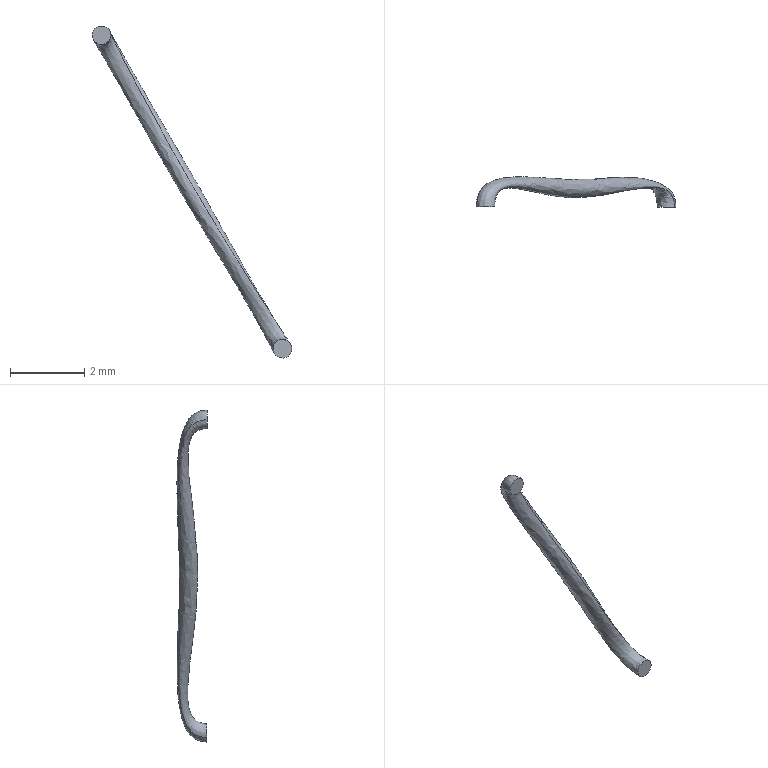Part | SolidWorks | features BaseBody 1 | 1 solid | 4 faces | box 5.38 x 0.8138 x 8.952 mm | volume 1.492 mm3 | plane 2 | spline 2
STEP:
#1=CARTESIAN_POINT('',(349.369,424.471,116.724));
#2=VERTEX_POINT('',#1);
#3=CARTESIAN_POINT('',(348.87,424.471,116.694));
#4=VERTEX_POINT('',#3);
#5=CARTESIAN_POINT('',(349.369,424.471,116.724));
#6=CARTESIAN_POINT('',(349.367,424.471,116.757));
#7=CARTESIAN_POINT('',(349.349,424.471,116.824));
#8=CARTESIAN_POINT('',(349.289,424.471,116.9));
#9=CARTESIAN_POINT('',(349.206,424.471,116.951));
#10=CARTESIAN_POINT('',(349.111,424.471,116.965));
#11=CARTESIAN_POINT('',(349.024,424.471,116.945));
#12=CARTESIAN_POINT('',(348.935,424.471,116.891));
#13=CARTESIAN_POINT('',(348.888,424.471,116.819));
#14=CARTESIAN_POINT('',(348.873,424.471,116.754));
#15=CARTESIAN_POINT('',(348.87,424.471,116.735));
#16=CARTESIAN_POINT('',(348.869,424.471,116.715));
#17=CARTESIAN_POINT('',(348.869,424.471,116.701));
#18=CARTESIAN_POINT('',(348.87,424.471,116.694));
#19=B_SPLINE_CURVE_WITH_KNOTS('',3,(#5,#6,#7,#8,#9,#10,#11,#12,#13,#14,#15,#16,#17,#18),.UNSPECIFIED.,.F.,.F.,(4,1,1,1,1,1,1,1,1,1,1,4),(0.,0.125,0.25,0.375,0.5,0.6,0.7,0.9,0.925,0.95,0.975,1.),.UNSPECIFIED.);
#20=EDGE_CURVE('',#2,#4,#19,.T.);
#21=ORIENTED_EDGE('',*,*,#20,.T.);
#22=CARTESIAN_POINT('',(348.87,424.471,116.694));
#23=CARTESIAN_POINT('',(348.87,424.471,116.687));
#24=CARTESIAN_POINT('',(348.872,424.471,116.674));
#25=CARTESIAN_POINT('',(348.875,424.471,116.654));
#26=CARTESIAN_POINT('',(348.88,424.471,116.634));
#27=CARTESIAN_POINT('',(348.903,424.471,116.572));
#28=CARTESIAN_POINT('',(348.958,424.471,116.506));
#29=CARTESIAN_POINT('',(349.053,424.471,116.464));
#30=CARTESIAN_POINT('',(349.142,424.471,116.454));
#31=CARTESIAN_POINT('',(349.234,424.471,116.479));
#32=CARTESIAN_POINT('',(349.311,424.471,116.539));
#33=CARTESIAN_POINT('',(349.361,424.471,116.623));
#34=CARTESIAN_POINT('',(349.371,424.471,116.69));
#35=CARTESIAN_POINT('',(349.369,424.471,116.724));
#36=B_SPLINE_CURVE_WITH_KNOTS('',3,(#22,#23,#24,#25,#26,#27,#28,#29,#30,#31,#32,#33,#34,#35),.UNSPECIFIED.,.F.,.F.,(4,1,1,1,1,1,1,1,1,1,1,4),(0.,0.025,0.05,0.075,0.1,0.3,0.4,0.5,0.625,0.75,0.875,1.),.UNSPECIFIED.);
#37=EDGE_CURVE('',#4,#2,#36,.T.);
#38=ORIENTED_EDGE('',*,*,#37,.T.);
#39=EDGE_LOOP('',(#21,#38));
#40=FACE_OUTER_BOUND('',#39,.T.);
#41=CARTESIAN_POINT('',(349.119,424.471,116.709));
#42=DIRECTION('',(-0.0009599,1.,0.));
#43=DIRECTION('',(0.,0.,1.));
#44=AXIS2_PLACEMENT_3D('',#41,#42,#43);
#45=PLANE('',#44);
#46=ADVANCED_FACE('',(#40),#45,.F.);
#47=CARTESIAN_POINT('',(354.216,424.476,108.382));
#48=VERTEX_POINT('',#47);
#49=CARTESIAN_POINT('',(353.783,424.475,108.132));
#50=VERTEX_POINT('',#49);
#51=CARTESIAN_POINT('',(354.216,424.476,108.382));
#52=CARTESIAN_POINT('',(354.199,424.476,108.411));
#53=CARTESIAN_POINT('',(354.153,424.476,108.462));
#54=CARTESIAN_POINT('',(354.065,424.476,108.504));
#55=CARTESIAN_POINT('',(353.968,424.476,108.512));
#56=CARTESIAN_POINT('',(353.877,424.476,108.482));
#57=CARTESIAN_POINT('',(353.809,424.475,108.425));
#58=CARTESIAN_POINT('',(353.753,424.475,108.337));
#59=CARTESIAN_POINT('',(353.743,424.475,108.251));
#60=CARTESIAN_POINT('',(353.759,424.475,108.188));
#61=CARTESIAN_POINT('',(353.765,424.475,108.169));
#62=CARTESIAN_POINT('',(353.773,424.475,108.15));
#63=CARTESIAN_POINT('',(353.779,424.475,108.138));
#64=CARTESIAN_POINT('',(353.783,424.475,108.132));
#65=B_SPLINE_CURVE_WITH_KNOTS('',3,(#51,#52,#53,#54,#55,#56,#57,#58,#59,#60,#61,#62,#63,#64),.UNSPECIFIED.,.F.,.F.,(4,1,1,1,1,1,1,1,1,1,1,4),(0.,0.125,0.25,0.375,0.5,0.6,0.7,0.9,0.925,0.95,0.975,1.),.UNSPECIFIED.);
#66=EDGE_CURVE('',#48,#50,#65,.T.);
#67=ORIENTED_EDGE('',*,*,#66,.T.);
#68=CARTESIAN_POINT('',(353.783,424.475,108.132));
#69=CARTESIAN_POINT('',(353.786,424.475,108.126));
#70=CARTESIAN_POINT('',(353.794,424.475,108.114));
#71=CARTESIAN_POINT('',(353.806,424.475,108.098));
#72=CARTESIAN_POINT('',(353.819,424.475,108.083));
#73=CARTESIAN_POINT('',(353.866,424.476,108.038));
#74=CARTESIAN_POINT('',(353.946,424.476,108.003));
#75=CARTESIAN_POINT('',(354.05,424.476,108.008));
#76=CARTESIAN_POINT('',(354.133,424.476,108.039));
#77=CARTESIAN_POINT('',(354.204,424.476,108.103));
#78=CARTESIAN_POINT('',(354.246,424.476,108.191));
#79=CARTESIAN_POINT('',(354.254,424.476,108.288));
#80=CARTESIAN_POINT('',(354.233,424.476,108.353));
#81=CARTESIAN_POINT('',(354.216,424.476,108.382));
#82=B_SPLINE_CURVE_WITH_KNOTS('',3,(#68,#69,#70,#71,#72,#73,#74,#75,#76,#77,#78,#79,#80,#81),.UNSPECIFIED.,.F.,.F.,(4,1,1,1,1,1,1,1,1,1,1,4),(0.,0.025,0.05,0.075,0.1,0.3,0.4,0.5,0.625,0.75,0.875,1.),.UNSPECIFIED.);
#83=EDGE_CURVE('',#50,#48,#82,.T.);
#84=ORIENTED_EDGE('',*,*,#83,.T.);
#85=EDGE_LOOP('',(#67,#84));
#86=FACE_OUTER_BOUND('',#85,.T.);
#87=CARTESIAN_POINT('',(353.999,424.476,108.257));
#88=DIRECTION('',(-0.0009599,1.,0.));
#89=DIRECTION('',(0.,0.,1.));
#90=AXIS2_PLACEMENT_3D('',#87,#88,#89);
#91=PLANE('',#90);
#92=ADVANCED_FACE('',(#86),#91,.F.);
#93=CARTESIAN_POINT('',(354.216,424.476,108.382));
#94=CARTESIAN_POINT('',(354.215,425.491,108.382));
#95=CARTESIAN_POINT('',(351.494,424.025,112.508));
#96=CARTESIAN_POINT('',(349.368,425.464,116.724));
#97=CARTESIAN_POINT('',(349.369,424.471,116.724));
#98=B_SPLINE_CURVE_WITH_KNOTS('',3,(#93,#94,#95,#96,#97),.UNSPECIFIED.,.F.,.F.,(4,1,4),(0.,0.5001,1.),.UNSPECIFIED.);
#99=EDGE_CURVE('',#48,#2,#98,.T.);
#100=ORIENTED_EDGE('',*,*,#99,.T.);
#101=ORIENTED_EDGE('',*,*,#37,.F.);
#102=CARTESIAN_POINT('',(348.87,424.471,116.694));
#103=CARTESIAN_POINT('',(348.869,425.576,116.694));
#104=CARTESIAN_POINT('',(351.562,424.823,112.419));
#105=CARTESIAN_POINT('',(353.782,425.559,108.132));
#106=CARTESIAN_POINT('',(353.783,424.475,108.132));
#107=B_SPLINE_CURVE_WITH_KNOTS('',3,(#102,#103,#104,#105,#106),.UNSPECIFIED.,.F.,.F.,(4,1,4),(0.,0.4999,1.),.UNSPECIFIED.);
#108=EDGE_CURVE('',#4,#50,#107,.T.);
#109=ORIENTED_EDGE('',*,*,#108,.T.);
#110=ORIENTED_EDGE('',*,*,#66,.F.);
#111=EDGE_LOOP('',(#100,#101,#109,#110));
#112=FACE_OUTER_BOUND('',#111,.T.);
#113=CARTESIAN_POINT('',(354.219,424.375,108.374));
#114=CARTESIAN_POINT('',(354.307,425.541,108.239));
#115=CARTESIAN_POINT('',(351.502,423.989,112.524));
#116=CARTESIAN_POINT('',(349.295,425.516,116.88));
#117=CARTESIAN_POINT('',(349.371,424.365,116.732));
#118=CARTESIAN_POINT('',(354.217,424.375,108.379));
#119=CARTESIAN_POINT('',(354.304,425.54,108.244));
#120=CARTESIAN_POINT('',(351.495,423.985,112.52));
#121=CARTESIAN_POINT('',(349.296,425.515,116.875));
#122=CARTESIAN_POINT('',(349.372,424.366,116.727));
#123=CARTESIAN_POINT('',(354.198,424.376,108.413));
#124=CARTESIAN_POINT('',(354.287,425.531,108.28));
#125=CARTESIAN_POINT('',(351.443,423.956,112.488));
#126=CARTESIAN_POINT('',(349.301,425.506,116.836));
#127=CARTESIAN_POINT('',(349.375,424.366,116.689));
#128=CARTESIAN_POINT('',(354.149,424.378,108.468));
#129=CARTESIAN_POINT('',(354.24,425.515,108.339));
#130=CARTESIAN_POINT('',(351.348,423.93,112.424));
#131=CARTESIAN_POINT('',(349.293,425.494,116.763));
#132=CARTESIAN_POINT('',(349.365,424.368,116.616));
#133=CARTESIAN_POINT('',(354.061,424.379,108.51));
#134=CARTESIAN_POINT('',(354.152,425.5,108.384));
#135=CARTESIAN_POINT('',(351.248,423.966,112.346));
#136=CARTESIAN_POINT('',(349.245,425.485,116.679));
#137=CARTESIAN_POINT('',(349.314,424.369,116.532));
#138=CARTESIAN_POINT('',(353.964,424.38,108.517));
#139=CARTESIAN_POINT('',(354.054,425.492,108.394));
#140=CARTESIAN_POINT('',(351.187,424.062,112.285));
#141=CARTESIAN_POINT('',(349.167,425.486,116.62));
#142=CARTESIAN_POINT('',(349.237,424.368,116.472));
#143=CARTESIAN_POINT('',(353.874,424.379,108.487));
#144=CARTESIAN_POINT('',(353.96,425.493,108.364));
#145=CARTESIAN_POINT('',(351.177,424.205,112.252));
#146=CARTESIAN_POINT('',(349.072,425.495,116.595));
#147=CARTESIAN_POINT('',(349.145,424.367,116.447));
#148=CARTESIAN_POINT('',(353.805,424.378,108.431));
#149=CARTESIAN_POINT('',(353.888,425.503,108.306));
#150=CARTESIAN_POINT('',(351.211,424.361,112.249));
#151=CARTESIAN_POINT('',(348.98,425.513,116.605));
#152=CARTESIAN_POINT('',(349.057,424.365,116.456));
#153=CARTESIAN_POINT('',(353.75,424.376,108.343));
#154=CARTESIAN_POINT('',(353.829,425.524,108.215));
#155=CARTESIAN_POINT('',(351.293,424.544,112.274));
#156=CARTESIAN_POINT('',(348.879,425.541,116.648));
#157=CARTESIAN_POINT('',(348.962,424.362,116.499));
#158=CARTESIAN_POINT('',(353.74,424.373,108.257));
#159=CARTESIAN_POINT('',(353.815,425.547,108.124));
#160=CARTESIAN_POINT('',(351.395,424.675,112.324));
#161=CARTESIAN_POINT('',(348.818,425.567,116.715));
#162=CARTESIAN_POINT('',(348.907,424.359,116.565));
#163=CARTESIAN_POINT('',(353.755,424.371,108.194));
#164=CARTESIAN_POINT('',(353.829,425.565,108.057));
#165=CARTESIAN_POINT('',(351.484,424.747,112.374));
#166=CARTESIAN_POINT('',(348.792,425.586,116.777));
#167=CARTESIAN_POINT('',(348.885,424.356,116.627));
#168=CARTESIAN_POINT('',(353.762,424.371,108.175));
#169=CARTESIAN_POINT('',(353.834,425.571,108.037));
#170=CARTESIAN_POINT('',(351.511,424.767,112.39));
#171=CARTESIAN_POINT('',(348.786,425.591,116.796));
#172=CARTESIAN_POINT('',(348.88,424.356,116.646));
#173=CARTESIAN_POINT('',(353.77,424.37,108.156));
#174=CARTESIAN_POINT('',(353.842,425.576,108.017));
#175=CARTESIAN_POINT('',(351.539,424.784,112.406));
#176=CARTESIAN_POINT('',(348.781,425.596,116.816));
#177=CARTESIAN_POINT('',(348.876,424.355,116.666));
#178=CARTESIAN_POINT('',(353.779,424.37,108.14));
#179=CARTESIAN_POINT('',(353.85,425.581,108.));
#180=CARTESIAN_POINT('',(351.564,424.798,112.422));
#181=CARTESIAN_POINT('',(348.779,425.601,116.835));
#182=CARTESIAN_POINT('',(348.874,424.355,116.685));
#183=CARTESIAN_POINT('',(353.785,424.37,108.129));
#184=CARTESIAN_POINT('',(353.856,425.585,107.989));
#185=CARTESIAN_POINT('',(351.581,424.806,112.433));
#186=CARTESIAN_POINT('',(348.778,425.604,116.847));
#187=CARTESIAN_POINT('',(348.874,424.355,116.697));
#188=CARTESIAN_POINT('',(353.788,424.369,108.125));
#189=CARTESIAN_POINT('',(353.859,425.586,107.984));
#190=CARTESIAN_POINT('',(351.588,424.809,112.437));
#191=CARTESIAN_POINT('',(348.777,425.605,116.853));
#192=CARTESIAN_POINT('',(348.874,424.354,116.702));
#193=B_SPLINE_SURFACE_WITH_KNOTS('',3,3,((#113,#114,#115,#116,#117),(#118,#119,#120,#121,#122),(#123,#124,#125,#126,#127),(#128,#129,#130,#131,#132),(#133,#134,#135,#136,#137),(#138,#139,#140,#141,#142),(#143,#144,#145,#146,#147),(#148,#149,#150,#151,#152),(#153,#154,#155,#156,#157),(#158,#159,#160,#161,#162),(#163,#164,#165,#166,#167),(#168,#169,#170,#171,#172),(#173,#174,#175,#176,#177),(#178,#179,#180,#181,#182),(#183,#184,#185,#186,#187),(#188,#189,#190,#191,#192)),.UNSPECIFIED.,.F.,.F.,.F.,(4,1,1,1,1,1,1,1,1,1,1,1,1,4),(4,1,4),(0.4905,0.5,0.5625,0.625,0.6875,0.75,0.8,0.85,0.95,0.9625,0.975,0.9875,1.,1.01),(-0.01559,0.5001,1.017),.UNSPECIFIED.);
#194=ADVANCED_FACE('',(#112),#193,.F.);
#195=ORIENTED_EDGE('',*,*,#83,.F.);
#196=ORIENTED_EDGE('',*,*,#108,.F.);
#197=ORIENTED_EDGE('',*,*,#20,.F.);
#198=ORIENTED_EDGE('',*,*,#99,.F.);
#199=EDGE_LOOP('',(#195,#196,#197,#198));
#200=FACE_OUTER_BOUND('',#199,.T.);
#201=CARTESIAN_POINT('',(353.772,424.37,108.152));
#202=CARTESIAN_POINT('',(353.844,425.578,108.013));
#203=CARTESIAN_POINT('',(351.545,424.788,112.41));
#204=CARTESIAN_POINT('',(348.781,425.598,116.821));
#205=CARTESIAN_POINT('',(348.876,424.355,116.671));
#206=CARTESIAN_POINT('',(353.774,424.37,108.147));
#207=CARTESIAN_POINT('',(353.846,425.579,108.008));
#208=CARTESIAN_POINT('',(351.552,424.792,112.415));
#209=CARTESIAN_POINT('',(348.78,425.599,116.826));
#210=CARTESIAN_POINT('',(348.875,424.355,116.676));
#211=CARTESIAN_POINT('',(353.78,424.37,108.137));
#212=CARTESIAN_POINT('',(353.851,425.582,107.997));
#213=CARTESIAN_POINT('',(351.569,424.8,112.425));
#214=CARTESIAN_POINT('',(348.778,425.602,116.839));
#215=CARTESIAN_POINT('',(348.874,424.355,116.688));
#216=CARTESIAN_POINT('',(353.79,424.369,108.121));
#217=CARTESIAN_POINT('',(353.861,425.587,107.98));
#218=CARTESIAN_POINT('',(351.594,424.812,112.441));
#219=CARTESIAN_POINT('',(348.777,425.606,116.858));
#220=CARTESIAN_POINT('',(348.874,424.354,116.707));
#221=CARTESIAN_POINT('',(353.803,424.369,108.105));
#222=CARTESIAN_POINT('',(353.873,425.592,107.962));
#223=CARTESIAN_POINT('',(351.621,424.821,112.459));
#224=CARTESIAN_POINT('',(348.777,425.611,116.878));
#225=CARTESIAN_POINT('',(348.875,424.354,116.727));
#226=CARTESIAN_POINT('',(353.816,424.368,108.09));
#227=CARTESIAN_POINT('',(353.886,425.597,107.947));
#228=CARTESIAN_POINT('',(351.647,424.828,112.476));
#229=CARTESIAN_POINT('',(348.779,425.615,116.898));
#230=CARTESIAN_POINT('',(348.878,424.353,116.747));
#231=CARTESIAN_POINT('',(353.863,424.367,108.044));
#232=CARTESIAN_POINT('',(353.932,425.612,107.898));
#233=CARTESIAN_POINT('',(351.729,424.84,112.533));
#234=CARTESIAN_POINT('',(348.792,425.626,116.962));
#235=CARTESIAN_POINT('',(348.893,424.352,116.811));
#236=CARTESIAN_POINT('',(353.943,424.366,108.01));
#237=CARTESIAN_POINT('',(354.011,425.625,107.86));
#238=CARTESIAN_POINT('',(351.814,424.802,112.601));
#239=CARTESIAN_POINT('',(348.838,425.632,117.035));
#240=CARTESIAN_POINT('',(348.94,424.352,116.884));
#241=CARTESIAN_POINT('',(354.046,424.366,108.014));
#242=CARTESIAN_POINT('',(354.117,425.628,107.863));
#243=CARTESIAN_POINT('',(351.864,424.685,112.658));
#244=CARTESIAN_POINT('',(348.928,425.627,117.088));
#245=CARTESIAN_POINT('',(349.029,424.353,116.937));
#246=CARTESIAN_POINT('',(354.13,424.367,108.046));
#247=CARTESIAN_POINT('',(354.203,425.624,107.894));
#248=CARTESIAN_POINT('',(351.869,424.55,112.685));
#249=CARTESIAN_POINT('',(349.018,425.615,117.108));
#250=CARTESIAN_POINT('',(349.116,424.354,116.957));
#251=CARTESIAN_POINT('',(354.201,424.368,108.11));
#252=CARTESIAN_POINT('',(354.277,425.611,107.96));
#253=CARTESIAN_POINT('',(351.826,424.382,112.685));
#254=CARTESIAN_POINT('',(349.117,425.594,117.093));
#255=CARTESIAN_POINT('',(349.21,424.357,116.943));
#256=CARTESIAN_POINT('',(354.243,424.371,108.197));
#257=CARTESIAN_POINT('',(354.323,425.588,108.052));
#258=CARTESIAN_POINT('',(351.738,424.215,112.653));
#259=CARTESIAN_POINT('',(349.206,425.566,117.043));
#260=CARTESIAN_POINT('',(349.293,424.36,116.893));
#261=CARTESIAN_POINT('',(354.25,424.373,108.294));
#262=CARTESIAN_POINT('',(354.335,425.562,108.154));
#263=CARTESIAN_POINT('',(351.62,424.071,112.594));
#264=CARTESIAN_POINT('',(349.272,425.537,116.965));
#265=CARTESIAN_POINT('',(349.353,424.363,116.816));
#266=CARTESIAN_POINT('',(354.227,424.375,108.364));
#267=CARTESIAN_POINT('',(354.314,425.544,108.228));
#268=CARTESIAN_POINT('',(351.52,423.996,112.536));
#269=CARTESIAN_POINT('',(349.295,425.519,116.894));
#270=CARTESIAN_POINT('',(349.372,424.365,116.745));
#271=CARTESIAN_POINT('',(354.207,424.376,108.397));
#272=CARTESIAN_POINT('',(354.295,425.535,108.263));
#273=CARTESIAN_POINT('',(351.468,423.971,112.503));
#274=CARTESIAN_POINT('',(349.298,425.511,116.855));
#275=CARTESIAN_POINT('',(349.373,424.366,116.707));
#276=CARTESIAN_POINT('',(354.204,424.376,108.401));
#277=CARTESIAN_POINT('',(354.292,425.534,108.267));
#278=CARTESIAN_POINT('',(351.461,423.968,112.498));
#279=CARTESIAN_POINT('',(349.298,425.51,116.85));
#280=CARTESIAN_POINT('',(349.373,424.366,116.701));
#281=B_SPLINE_SURFACE_WITH_KNOTS('',3,3,((#201,#202,#203,#204,#205),(#206,#207,#208,#209,#210),(#211,#212,#213,#214,#215),(#216,#217,#218,#219,#220),(#221,#222,#223,#224,#225),(#226,#227,#228,#229,#230),(#231,#232,#233,#234,#235),(#236,#237,#238,#239,#240),(#241,#242,#243,#244,#245),(#246,#247,#248,#249,#250),(#251,#252,#253,#254,#255),(#256,#257,#258,#259,#260),(#261,#262,#263,#264,#265),(#266,#267,#268,#269,#270),(#271,#272,#273,#274,#275),(#276,#277,#278,#279,#280)),.UNSPECIFIED.,.F.,.F.,.F.,(4,1,1,1,1,1,1,1,1,1,1,1,1,4),(4,1,4),(-0.009538,0.,0.0125,0.025,0.0375,0.05,0.15,0.2,0.25,0.3125,0.375,0.4375,0.5,0.5095),(-0.01559,0.5001,1.017),.UNSPECIFIED.);
#282=ADVANCED_FACE('',(#200),#281,.F.);
#283=CLOSED_SHELL('',(#46,#92,#194,#282));
#284=MANIFOLD_SOLID_BREP('',#283);
#285=CARTESIAN_POINT('',(0.,0.,0.));
#286=DIRECTION('',(0.,0.,1.));
#287=DIRECTION('',(1.,0.,0.));
#288=AXIS2_PLACEMENT_3D('',#285,#286,#287);
#289=(LENGTH_UNIT()NAMED_UNIT(*)SI_UNIT(.MILLI.,.METRE.));
#290=UNCERTAINTY_MEASURE_WITH_UNIT(LENGTH_MEASURE(0.00001),#289,'','');
#291=(NAMED_UNIT(*)PLANE_ANGLE_UNIT()SI_UNIT($,.RADIAN.));
#292=(NAMED_UNIT(*)SI_UNIT($,.STERADIAN.)SOLID_ANGLE_UNIT());
#293=(GEOMETRIC_REPRESENTATION_CONTEXT(3)GLOBAL_UNCERTAINTY_ASSIGNED_CONTEXT((#290))GLOBAL_UNIT_ASSIGNED_CONTEXT((#289,#291,#292))REPRESENTATION_CONTEXT('',''));
#294=ADVANCED_BREP_SHAPE_REPRESENTATION('',(#284,#288),#293);